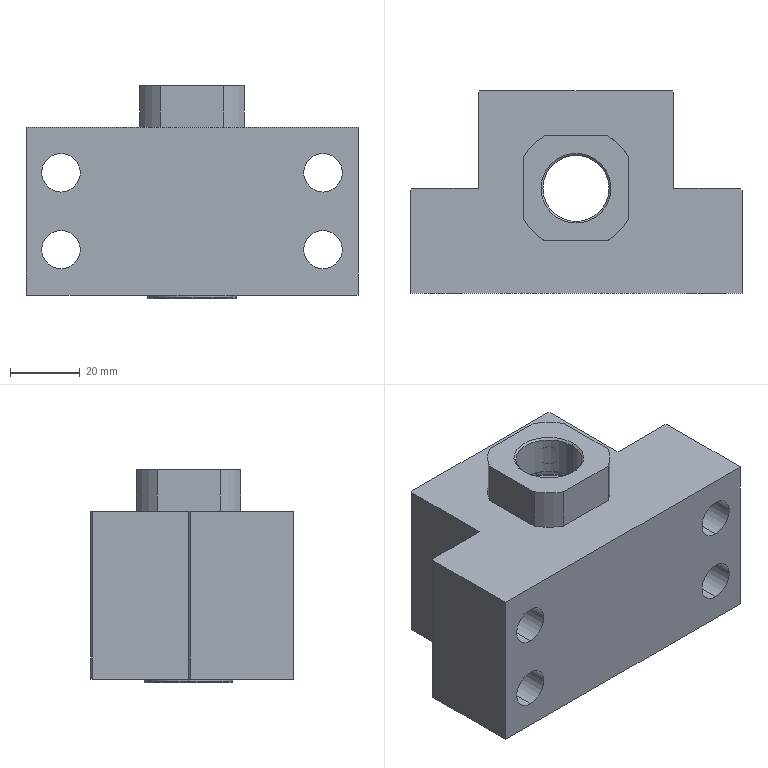Part | STEP file | LEB23-20 | 1 solid | 128 faces | box 95 x 58 x 61 mm | volume 169444 mm3 | cylinder 56 | plane 36 | spline 28 | cone 8 | commonest cylinder face diameters 11 x8 17 x8 20 x6 26 x6 47 x6 29.2 x4